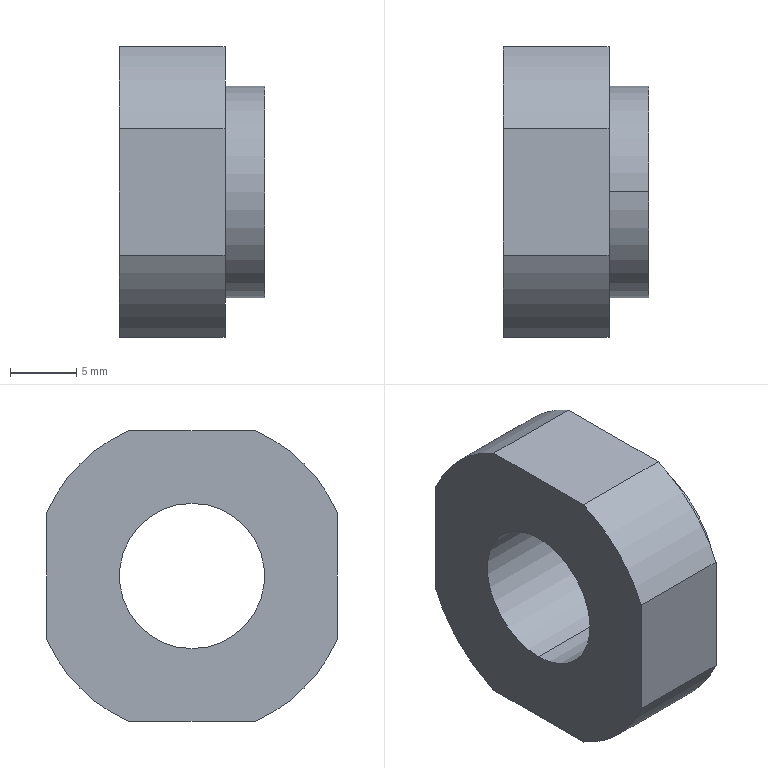Part | STEP file | PN_0032 locking nut | 1 solid | 15 faces | box 11 x 22 x 22 mm | volume 2971 mm3 | cylinder 8 | plane 7 | commonest cylinder face diameters 24 x4 11 x2 16 x2
STEP:
#1=CARTESIAN_POINT('',(0.,0.,0.));
#2=DIRECTION('',(0.,0.,1.));
#3=DIRECTION('',(1.,0.,0.));
#4=AXIS2_PLACEMENT_3D('',#1,#2,#3);
#5=CARTESIAN_POINT('',(-11.,0.,-5.5));
#6=VERTEX_POINT('',#5);
#7=CARTESIAN_POINT('',(0.,0.,-5.5));
#8=VERTEX_POINT('',#7);
#9=CARTESIAN_POINT('',(-11.,0.,-5.5));
#10=DIRECTION('',(1.,0.,0.));
#11=VECTOR('',#10,1.);
#12=LINE('',#9,#11);
#13=CARTESIAN_POINT('',(-11.,0.,0.));
#14=DIRECTION('',(1.,0.,0.));
#15=DIRECTION('',(0.,0.,-1.));
#16=AXIS2_PLACEMENT_3D('',#13,#14,#15);
#17=CYLINDRICAL_SURFACE('',#16,5.5);
#18=CARTESIAN_POINT('',(6.283,0.));
#19=DIRECTION('',(0.,1.));
#20=VECTOR('',#19,1.);
#21=LINE('',#18,#20);
#22=(GEOMETRIC_REPRESENTATION_CONTEXT(2)PARAMETRIC_REPRESENTATION_CONTEXT()REPRESENTATION_CONTEXT('',''));
#23=DEFINITIONAL_REPRESENTATION('',(#21),#22);
#24=PCURVE('',#17,#23);
#25=CARTESIAN_POINT('',(-11.,0.,0.));
#26=DIRECTION('',(1.,0.,0.));
#27=DIRECTION('',(0.,0.,-1.));
#28=AXIS2_PLACEMENT_3D('',#25,#26,#27);
#29=CYLINDRICAL_SURFACE('',#28,5.5);
#30=CARTESIAN_POINT('',(0.,0.));
#31=DIRECTION('',(0.,1.));
#32=VECTOR('',#31,1.);
#33=LINE('',#30,#32);
#34=(GEOMETRIC_REPRESENTATION_CONTEXT(2)PARAMETRIC_REPRESENTATION_CONTEXT()REPRESENTATION_CONTEXT('',''));
#35=DEFINITIONAL_REPRESENTATION('',(#33),#34);
#36=PCURVE('',#29,#35);
#37=SURFACE_CURVE('',#12,(#24,#36),.PCURVE_S1.);
#38=EDGE_CURVE('',#6,#8,#37,.T.);
#39=ORIENTED_EDGE('',*,*,#38,.T.);
#40=CARTESIAN_POINT('',(0.,0.,5.5));
#41=VERTEX_POINT('',#40);
#42=CARTESIAN_POINT('',(0.,0.,0.));
#43=DIRECTION('',(1.,0.,0.));
#44=DIRECTION('',(0.,0.,-1.));
#45=AXIS2_PLACEMENT_3D('',#42,#43,#44);
#46=CIRCLE('',#45,5.5);
#47=CARTESIAN_POINT('',(0.,11.));
#48=DIRECTION('',(1.,0.));
#49=VECTOR('',#48,1.);
#50=LINE('',#47,#49);
#51=(GEOMETRIC_REPRESENTATION_CONTEXT(2)PARAMETRIC_REPRESENTATION_CONTEXT()REPRESENTATION_CONTEXT('',''));
#52=DEFINITIONAL_REPRESENTATION('',(#50),#51);
#53=PCURVE('',#17,#52);
#54=CARTESIAN_POINT('',(0.,0.,0.));
#55=DIRECTION('',(1.,0.,0.));
#56=DIRECTION('',(0.,0.,-1.));
#57=AXIS2_PLACEMENT_3D('',#54,#55,#56);
#58=PLANE('',#57);
#59=CARTESIAN_POINT('',(0.,0.));
#60=DIRECTION('',(1.,0.));
#61=AXIS2_PLACEMENT_2D('',#59,#60);
#62=CIRCLE('',#61,5.5);
#63=(GEOMETRIC_REPRESENTATION_CONTEXT(2)PARAMETRIC_REPRESENTATION_CONTEXT()REPRESENTATION_CONTEXT('',''));
#64=DEFINITIONAL_REPRESENTATION('',(#62),#63);
#65=PCURVE('',#58,#64);
#66=SURFACE_CURVE('',#46,(#53,#65),.PCURVE_S1.);
#67=EDGE_CURVE('',#41,#8,#66,.T.);
#68=ORIENTED_EDGE('',*,*,#67,.F.);
#69=CARTESIAN_POINT('',(-11.,0.,5.5));
#70=VERTEX_POINT('',#69);
#71=CARTESIAN_POINT('',(-11.,0.,5.5));
#72=DIRECTION('',(1.,0.,0.));
#73=VECTOR('',#72,1.);
#74=LINE('',#71,#73);
#75=CARTESIAN_POINT('',(3.142,0.));
#76=DIRECTION('',(0.,1.));
#77=VECTOR('',#76,1.);
#78=LINE('',#75,#77);
#79=(GEOMETRIC_REPRESENTATION_CONTEXT(2)PARAMETRIC_REPRESENTATION_CONTEXT()REPRESENTATION_CONTEXT('',''));
#80=DEFINITIONAL_REPRESENTATION('',(#78),#79);
#81=PCURVE('',#17,#80);
#82=CARTESIAN_POINT('',(3.142,0.));
#83=DIRECTION('',(0.,1.));
#84=VECTOR('',#83,1.);
#85=LINE('',#82,#84);
#86=(GEOMETRIC_REPRESENTATION_CONTEXT(2)PARAMETRIC_REPRESENTATION_CONTEXT()REPRESENTATION_CONTEXT('',''));
#87=DEFINITIONAL_REPRESENTATION('',(#85),#86);
#88=PCURVE('',#29,#87);
#89=SURFACE_CURVE('',#74,(#81,#88),.PCURVE_S1.);
#90=EDGE_CURVE('',#70,#41,#89,.T.);
#91=ORIENTED_EDGE('',*,*,#90,.F.);
#92=CARTESIAN_POINT('',(-11.,0.,0.));
#93=DIRECTION('',(1.,0.,0.));
#94=DIRECTION('',(0.,0.,-1.));
#95=AXIS2_PLACEMENT_3D('',#92,#93,#94);
#96=CIRCLE('',#95,5.5);
#97=CARTESIAN_POINT('',(0.,0.));
#98=DIRECTION('',(1.,0.));
#99=VECTOR('',#98,1.);
#100=LINE('',#97,#99);
#101=(GEOMETRIC_REPRESENTATION_CONTEXT(2)PARAMETRIC_REPRESENTATION_CONTEXT()REPRESENTATION_CONTEXT('',''));
#102=DEFINITIONAL_REPRESENTATION('',(#100),#101);
#103=PCURVE('',#17,#102);
#104=CARTESIAN_POINT('',(-11.,12.,0.));
#105=DIRECTION('',(-1.,0.,0.));
#106=DIRECTION('',(0.,0.,1.));
#107=AXIS2_PLACEMENT_3D('',#104,#105,#106);
#108=PLANE('',#107);
#109=CARTESIAN_POINT('',(-5.5,-12.));
#110=CARTESIAN_POINT('',(-5.5,-2.474));
#111=CARTESIAN_POINT('',(2.75,-7.237));
#112=CARTESIAN_POINT('',(11.,-12.));
#113=CARTESIAN_POINT('',(2.75,-16.763));
#114=CARTESIAN_POINT('',(-5.5,-21.526));
#115=CARTESIAN_POINT('',(-5.5,-12.));
#116=(BOUNDED_CURVE()B_SPLINE_CURVE(2,(#109,#110,#111,#112,#113,#114,#115),.UNSPECIFIED.,.T.,.F.)B_SPLINE_CURVE_WITH_KNOTS((1,2,2,2,2,1),(-2.094,0.,2.094,4.189,6.283,8.378),.UNSPECIFIED.)CURVE()GEOMETRIC_REPRESENTATION_ITEM()RATIONAL_B_SPLINE_CURVE((1.,0.5,1.,0.5,1.,0.5,1.))REPRESENTATION_ITEM(''));
#117=(GEOMETRIC_REPRESENTATION_CONTEXT(2)PARAMETRIC_REPRESENTATION_CONTEXT()REPRESENTATION_CONTEXT('',''));
#118=DEFINITIONAL_REPRESENTATION('',(#116),#117);
#119=PCURVE('',#108,#118);
#120=SURFACE_CURVE('',#96,(#103,#119),.PCURVE_S1.);
#121=EDGE_CURVE('',#70,#6,#120,.T.);
#122=ORIENTED_EDGE('',*,*,#121,.T.);
#123=EDGE_LOOP('',(#39,#68,#91,#122));
#124=FACE_BOUND('',#123,.F.);
#125=ADVANCED_FACE('',(#124),#17,.F.);
#126=CARTESIAN_POINT('',(-3.,0.,-8.));
#127=VERTEX_POINT('',#126);
#128=CARTESIAN_POINT('',(-3.,0.,8.));
#129=VERTEX_POINT('',#128);
#130=CARTESIAN_POINT('',(-3.,0.,0.));
#131=DIRECTION('',(1.,0.,0.));
#132=DIRECTION('',(0.,0.,-1.));
#133=AXIS2_PLACEMENT_3D('',#130,#131,#132);
#134=CIRCLE('',#133,8.);
#135=CARTESIAN_POINT('',(0.,0.,0.));
#136=DIRECTION('',(1.,0.,0.));
#137=DIRECTION('',(0.,0.,-1.));
#138=AXIS2_PLACEMENT_3D('',#135,#136,#137);
#139=CYLINDRICAL_SURFACE('',#138,8.);
#140=CARTESIAN_POINT('',(0.,-3.));
#141=DIRECTION('',(1.,0.));
#142=VECTOR('',#141,1.);
#143=LINE('',#140,#142);
#144=(GEOMETRIC_REPRESENTATION_CONTEXT(2)PARAMETRIC_REPRESENTATION_CONTEXT()REPRESENTATION_CONTEXT('',''));
#145=DEFINITIONAL_REPRESENTATION('',(#143),#144);
#146=PCURVE('',#139,#145);
#147=CARTESIAN_POINT('',(-3.,8.,0.));
#148=DIRECTION('',(1.,0.,0.));
#149=DIRECTION('',(0.,0.,-1.));
#150=AXIS2_PLACEMENT_3D('',#147,#148,#149);
#151=PLANE('',#150);
#152=CARTESIAN_POINT('',(0.,-8.));
#153=DIRECTION('',(1.,0.));
#154=AXIS2_PLACEMENT_2D('',#152,#153);
#155=CIRCLE('',#154,8.);
#156=(GEOMETRIC_REPRESENTATION_CONTEXT(2)PARAMETRIC_REPRESENTATION_CONTEXT()REPRESENTATION_CONTEXT('',''));
#157=DEFINITIONAL_REPRESENTATION('',(#155),#156);
#158=PCURVE('',#151,#157);
#159=SURFACE_CURVE('',#134,(#146,#158),.PCURVE_S1.);
#160=EDGE_CURVE('',#127,#129,#159,.T.);
#161=ORIENTED_EDGE('',*,*,#160,.T.);
#162=CARTESIAN_POINT('',(0.,0.,8.));
#163=VERTEX_POINT('',#162);
#164=CARTESIAN_POINT('',(0.,0.,8.));
#165=DIRECTION('',(1.,0.,0.));
#166=VECTOR('',#165,1.);
#167=LINE('',#164,#166);
#168=CARTESIAN_POINT('',(3.142,0.));
#169=DIRECTION('',(0.,1.));
#170=VECTOR('',#169,1.);
#171=LINE('',#168,#170);
#172=(GEOMETRIC_REPRESENTATION_CONTEXT(2)PARAMETRIC_REPRESENTATION_CONTEXT()REPRESENTATION_CONTEXT('',''));
#173=DEFINITIONAL_REPRESENTATION('',(#171),#172);
#174=PCURVE('',#139,#173);
#175=CARTESIAN_POINT('',(0.,0.,0.));
#176=DIRECTION('',(1.,0.,0.));
#177=DIRECTION('',(0.,0.,-1.));
#178=AXIS2_PLACEMENT_3D('',#175,#176,#177);
#179=CYLINDRICAL_SURFACE('',#178,8.);
#180=CARTESIAN_POINT('',(3.142,0.));
#181=DIRECTION('',(0.,1.));
#182=VECTOR('',#181,1.);
#183=LINE('',#180,#182);
#184=(GEOMETRIC_REPRESENTATION_CONTEXT(2)PARAMETRIC_REPRESENTATION_CONTEXT()REPRESENTATION_CONTEXT('',''));
#185=DEFINITIONAL_REPRESENTATION('',(#183),#184);
#186=PCURVE('',#179,#185);
#187=SURFACE_CURVE('',#167,(#174,#186),.PCURVE_S1.);
#188=EDGE_CURVE('',#129,#163,#187,.T.);
#189=ORIENTED_EDGE('',*,*,#188,.T.);
#190=CARTESIAN_POINT('',(0.,0.,-8.));
#191=VERTEX_POINT('',#190);
#192=CARTESIAN_POINT('',(0.,0.,0.));
#193=DIRECTION('',(1.,0.,0.));
#194=DIRECTION('',(0.,0.,-1.));
#195=AXIS2_PLACEMENT_3D('',#192,#193,#194);
#196=CIRCLE('',#195,8.);
#197=CARTESIAN_POINT('',(0.,0.));
#198=DIRECTION('',(1.,0.));
#199=VECTOR('',#198,1.);
#200=LINE('',#197,#199);
#201=(GEOMETRIC_REPRESENTATION_CONTEXT(2)PARAMETRIC_REPRESENTATION_CONTEXT()REPRESENTATION_CONTEXT('',''));
#202=DEFINITIONAL_REPRESENTATION('',(#200),#201);
#203=PCURVE('',#139,#202);
#204=CARTESIAN_POINT('',(0.,0.));
#205=DIRECTION('',(1.,0.));
#206=AXIS2_PLACEMENT_2D('',#204,#205);
#207=CIRCLE('',#206,8.);
#208=(GEOMETRIC_REPRESENTATION_CONTEXT(2)PARAMETRIC_REPRESENTATION_CONTEXT()REPRESENTATION_CONTEXT('',''));
#209=DEFINITIONAL_REPRESENTATION('',(#207),#208);
#210=PCURVE('',#58,#209);
#211=SURFACE_CURVE('',#196,(#203,#210),.PCURVE_S1.);
#212=EDGE_CURVE('',#191,#163,#211,.T.);
#213=ORIENTED_EDGE('',*,*,#212,.F.);
#214=CARTESIAN_POINT('',(0.,0.,-8.));
#215=DIRECTION('',(1.,0.,0.));
#216=VECTOR('',#215,1.);
#217=LINE('',#214,#216);
#218=CARTESIAN_POINT('',(0.,0.));
#219=DIRECTION('',(0.,1.));
#220=VECTOR('',#219,1.);
#221=LINE('',#218,#220);
#222=(GEOMETRIC_REPRESENTATION_CONTEXT(2)PARAMETRIC_REPRESENTATION_CONTEXT()REPRESENTATION_CONTEXT('',''));
#223=DEFINITIONAL_REPRESENTATION('',(#221),#222);
#224=PCURVE('',#139,#223);
#225=CARTESIAN_POINT('',(6.283,0.));
#226=DIRECTION('',(0.,1.));
#227=VECTOR('',#226,1.);
#228=LINE('',#225,#227);
#229=(GEOMETRIC_REPRESENTATION_CONTEXT(2)PARAMETRIC_REPRESENTATION_CONTEXT()REPRESENTATION_CONTEXT('',''));
#230=DEFINITIONAL_REPRESENTATION('',(#228),#229);
#231=PCURVE('',#179,#230);
#232=SURFACE_CURVE('',#217,(#224,#231),.PCURVE_S1.);
#233=EDGE_CURVE('',#127,#191,#232,.T.);
#234=ORIENTED_EDGE('',*,*,#233,.F.);
#235=EDGE_LOOP('',(#161,#189,#213,#234));
#236=FACE_BOUND('',#235,.T.);
#237=ADVANCED_FACE('',(#236),#139,.T.);
#238=CARTESIAN_POINT('',(-3.,4.796,11.));
#239=VERTEX_POINT('',#238);
#240=CARTESIAN_POINT('',(-11.,4.796,11.));
#241=VERTEX_POINT('',#240);
#242=CARTESIAN_POINT('',(0.,4.796,11.));
#243=DIRECTION('',(-1.,0.,0.));
#244=VECTOR('',#243,1.);
#245=LINE('',#242,#244);
#246=CARTESIAN_POINT('',(0.,0.,0.));
#247=DIRECTION('',(1.,0.,0.));
#248=DIRECTION('',(0.,0.,-1.));
#249=AXIS2_PLACEMENT_3D('',#246,#247,#248);
#250=CYLINDRICAL_SURFACE('',#249,12.);
#251=CARTESIAN_POINT('',(2.73,0.));
#252=DIRECTION('',(0.,-1.));
#253=VECTOR('',#252,1.);
#254=LINE('',#251,#253);
#255=(GEOMETRIC_REPRESENTATION_CONTEXT(2)PARAMETRIC_REPRESENTATION_CONTEXT()REPRESENTATION_CONTEXT('',''));
#256=DEFINITIONAL_REPRESENTATION('',(#254),#255);
#257=PCURVE('',#250,#256);
#258=CARTESIAN_POINT('',(0.,17.205,11.));
#259=DIRECTION('',(0.,0.,-1.));
#260=DIRECTION('',(0.,1.,0.));
#261=AXIS2_PLACEMENT_3D('',#258,#259,#260);
#262=PLANE('',#261);
#263=CARTESIAN_POINT('',(-12.409,0.));
#264=DIRECTION('',(0.,-1.));
#265=VECTOR('',#264,1.);
#266=LINE('',#263,#265);
#267=(GEOMETRIC_REPRESENTATION_CONTEXT(2)PARAMETRIC_REPRESENTATION_CONTEXT()REPRESENTATION_CONTEXT('',''));
#268=DEFINITIONAL_REPRESENTATION('',(#266),#267);
#269=PCURVE('',#262,#268);
#270=SURFACE_CURVE('',#245,(#257,#269),.PCURVE_S1.);
#271=EDGE_CURVE('',#239,#241,#270,.T.);
#272=ORIENTED_EDGE('',*,*,#271,.F.);
#273=CARTESIAN_POINT('',(-3.,11.,4.796));
#274=VERTEX_POINT('',#273);
#275=CARTESIAN_POINT('',(-3.,0.,0.));
#276=DIRECTION('',(1.,0.,0.));
#277=DIRECTION('',(0.,0.,-1.));
#278=AXIS2_PLACEMENT_3D('',#275,#276,#277);
#279=CIRCLE('',#278,12.);
#280=CARTESIAN_POINT('',(0.,-3.));
#281=DIRECTION('',(1.,0.));
#282=VECTOR('',#281,1.);
#283=LINE('',#280,#282);
#284=(GEOMETRIC_REPRESENTATION_CONTEXT(2)PARAMETRIC_REPRESENTATION_CONTEXT()REPRESENTATION_CONTEXT('',''));
#285=DEFINITIONAL_REPRESENTATION('',(#283),#284);
#286=PCURVE('',#250,#285);
#287=CARTESIAN_POINT('',(0.,-8.));
#288=DIRECTION('',(1.,0.));
#289=AXIS2_PLACEMENT_2D('',#287,#288);
#290=CIRCLE('',#289,12.);
#291=(GEOMETRIC_REPRESENTATION_CONTEXT(2)PARAMETRIC_REPRESENTATION_CONTEXT()REPRESENTATION_CONTEXT('',''));
#292=DEFINITIONAL_REPRESENTATION('',(#290),#291);
#293=PCURVE('',#151,#292);
#294=SURFACE_CURVE('',#279,(#286,#293),.PCURVE_S1.);
#295=EDGE_CURVE('',#274,#239,#294,.T.);
#296=ORIENTED_EDGE('',*,*,#295,.F.);
#297=CARTESIAN_POINT('',(-11.,11.,4.796));
#298=VERTEX_POINT('',#297);
#299=CARTESIAN_POINT('',(0.,11.,4.796));
#300=DIRECTION('',(1.,0.,0.));
#301=VECTOR('',#300,1.);
#302=LINE('',#299,#301);
#303=CARTESIAN_POINT('',(1.982,0.));
#304=DIRECTION('',(0.,1.));
#305=VECTOR('',#304,1.);
#306=LINE('',#303,#305);
#307=(GEOMETRIC_REPRESENTATION_CONTEXT(2)PARAMETRIC_REPRESENTATION_CONTEXT()REPRESENTATION_CONTEXT('',''));
#308=DEFINITIONAL_REPRESENTATION('',(#306),#307);
#309=PCURVE('',#250,#308);
#310=CARTESIAN_POINT('',(0.,11.,-20.296));
#311=DIRECTION('',(0.,-1.,0.));
#312=DIRECTION('',(0.,0.,-1.));
#313=AXIS2_PLACEMENT_3D('',#310,#311,#312);
#314=PLANE('',#313);
#315=CARTESIAN_POINT('',(-25.092,0.));
#316=DIRECTION('',(0.,1.));
#317=VECTOR('',#316,1.);
#318=LINE('',#315,#317);
#319=(GEOMETRIC_REPRESENTATION_CONTEXT(2)PARAMETRIC_REPRESENTATION_CONTEXT()REPRESENTATION_CONTEXT('',''));
#320=DEFINITIONAL_REPRESENTATION('',(#318),#319);
#321=PCURVE('',#314,#320);
#322=SURFACE_CURVE('',#302,(#309,#321),.PCURVE_S1.);
#323=EDGE_CURVE('',#298,#274,#322,.T.);
#324=ORIENTED_EDGE('',*,*,#323,.F.);
#325=CARTESIAN_POINT('',(-11.,0.,0.));
#326=DIRECTION('',(1.,0.,0.));
#327=DIRECTION('',(0.,0.,-1.));
#328=AXIS2_PLACEMENT_3D('',#325,#326,#327);
#329=CIRCLE('',#328,12.);
#330=CARTESIAN_POINT('',(0.,-11.));
#331=DIRECTION('',(1.,0.));
#332=VECTOR('',#331,1.);
#333=LINE('',#330,#332);
#334=(GEOMETRIC_REPRESENTATION_CONTEXT(2)PARAMETRIC_REPRESENTATION_CONTEXT()REPRESENTATION_CONTEXT('',''));
#335=DEFINITIONAL_REPRESENTATION('',(#333),#334);
#336=PCURVE('',#250,#335);
#337=CARTESIAN_POINT('',(-12.,-12.));
#338=CARTESIAN_POINT('',(-12.,8.785));
#339=CARTESIAN_POINT('',(6.,-1.608));
#340=CARTESIAN_POINT('',(24.,-12.));
#341=CARTESIAN_POINT('',(6.,-22.392));
#342=CARTESIAN_POINT('',(-12.,-32.785));
#343=CARTESIAN_POINT('',(-12.,-12.));
#344=(BOUNDED_CURVE()B_SPLINE_CURVE(2,(#337,#338,#339,#340,#341,#342,#343),.UNSPECIFIED.,.T.,.F.)B_SPLINE_CURVE_WITH_KNOTS((1,2,2,2,2,1),(-2.094,0.,2.094,4.189,6.283,8.378),.UNSPECIFIED.)CURVE()GEOMETRIC_REPRESENTATION_ITEM()RATIONAL_B_SPLINE_CURVE((1.,0.5,1.,0.5,1.,0.5,1.))REPRESENTATION_ITEM(''));
#345=(GEOMETRIC_REPRESENTATION_CONTEXT(2)PARAMETRIC_REPRESENTATION_CONTEXT()REPRESENTATION_CONTEXT('',''));
#346=DEFINITIONAL_REPRESENTATION('',(#344),#345);
#347=PCURVE('',#108,#346);
#348=SURFACE_CURVE('',#329,(#336,#347),.PCURVE_S1.);
#349=EDGE_CURVE('',#298,#241,#348,.T.);
#350=ORIENTED_EDGE('',*,*,#349,.T.);
#351=EDGE_LOOP('',(#272,#296,#324,#350));
#352=FACE_BOUND('',#351,.T.);
#353=ADVANCED_FACE('',(#352),#250,.T.);
#354=CARTESIAN_POINT('',(-3.,-4.796,-11.));
#355=VERTEX_POINT('',#354);
#356=CARTESIAN_POINT('',(-11.,-4.796,-11.));
#357=VERTEX_POINT('',#356);
#358=CARTESIAN_POINT('',(0.,-4.796,-11.));
#359=DIRECTION('',(-1.,0.,0.));
#360=VECTOR('',#359,1.);
#361=LINE('',#358,#360);
#362=CARTESIAN_POINT('',(0.,0.,0.));
#363=DIRECTION('',(1.,0.,0.));
#364=DIRECTION('',(0.,0.,-1.));
#365=AXIS2_PLACEMENT_3D('',#362,#363,#364);
#366=CYLINDRICAL_SURFACE('',#365,12.);
#367=CARTESIAN_POINT('',(5.872,0.));
#368=DIRECTION('',(0.,-1.));
#369=VECTOR('',#368,1.);
#370=LINE('',#367,#369);
#371=(GEOMETRIC_REPRESENTATION_CONTEXT(2)PARAMETRIC_REPRESENTATION_CONTEXT()REPRESENTATION_CONTEXT('',''));
#372=DEFINITIONAL_REPRESENTATION('',(#370),#371);
#373=PCURVE('',#366,#372);
#374=CARTESIAN_POINT('',(0.,17.205,-11.));
#375=DIRECTION('',(0.,0.,1.));
#376=DIRECTION('',(0.,-1.,0.));
#377=AXIS2_PLACEMENT_3D('',#374,#375,#376);
#378=PLANE('',#377);
#379=CARTESIAN_POINT('',(22.001,0.));
#380=DIRECTION('',(0.,-1.));
#381=VECTOR('',#380,1.);
#382=LINE('',#379,#381);
#383=(GEOMETRIC_REPRESENTATION_CONTEXT(2)PARAMETRIC_REPRESENTATION_CONTEXT()REPRESENTATION_CONTEXT('',''));
#384=DEFINITIONAL_REPRESENTATION('',(#382),#383);
#385=PCURVE('',#378,#384);
#386=SURFACE_CURVE('',#361,(#373,#385),.PCURVE_S1.);
#387=EDGE_CURVE('',#355,#357,#386,.T.);
#388=ORIENTED_EDGE('',*,*,#387,.F.);
#389=CARTESIAN_POINT('',(-3.,-11.,-4.796));
#390=VERTEX_POINT('',#389);
#391=CARTESIAN_POINT('',(-3.,0.,0.));
#392=DIRECTION('',(1.,0.,0.));
#393=DIRECTION('',(0.,0.,-1.));
#394=AXIS2_PLACEMENT_3D('',#391,#392,#393);
#395=CIRCLE('',#394,12.);
#396=CARTESIAN_POINT('',(0.,-3.));
#397=DIRECTION('',(1.,0.));
#398=VECTOR('',#397,1.);
#399=LINE('',#396,#398);
#400=(GEOMETRIC_REPRESENTATION_CONTEXT(2)PARAMETRIC_REPRESENTATION_CONTEXT()REPRESENTATION_CONTEXT('',''));
#401=DEFINITIONAL_REPRESENTATION('',(#399),#400);
#402=PCURVE('',#366,#401);
#403=CARTESIAN_POINT('',(0.,-8.));
#404=DIRECTION('',(1.,0.));
#405=AXIS2_PLACEMENT_2D('',#403,#404);
#406=CIRCLE('',#405,12.);
#407=(GEOMETRIC_REPRESENTATION_CONTEXT(2)PARAMETRIC_REPRESENTATION_CONTEXT()REPRESENTATION_CONTEXT('',''));
#408=DEFINITIONAL_REPRESENTATION('',(#406),#407);
#409=PCURVE('',#151,#408);
#410=SURFACE_CURVE('',#395,(#402,#409),.PCURVE_S1.);
#411=EDGE_CURVE('',#390,#355,#410,.T.);
#412=ORIENTED_EDGE('',*,*,#411,.F.);
#413=CARTESIAN_POINT('',(-11.,-11.,-4.796));
#414=VERTEX_POINT('',#413);
#415=CARTESIAN_POINT('',(0.,-11.,-4.796));
#416=DIRECTION('',(1.,0.,0.));
#417=VECTOR('',#416,1.);
#418=LINE('',#415,#417);
#419=CARTESIAN_POINT('',(5.124,0.));
#420=DIRECTION('',(0.,1.));
#421=VECTOR('',#420,1.);
#422=LINE('',#419,#421);
#423=(GEOMETRIC_REPRESENTATION_CONTEXT(2)PARAMETRIC_REPRESENTATION_CONTEXT()REPRESENTATION_CONTEXT('',''));
#424=DEFINITIONAL_REPRESENTATION('',(#422),#423);
#425=PCURVE('',#366,#424);
#426=CARTESIAN_POINT('',(0.,-11.,-20.296));
#427=DIRECTION('',(0.,1.,0.));
#428=DIRECTION('',(0.,0.,1.));
#429=AXIS2_PLACEMENT_3D('',#426,#427,#428);
#430=PLANE('',#429);
#431=CARTESIAN_POINT('',(15.501,0.));
#432=DIRECTION('',(0.,1.));
#433=VECTOR('',#432,1.);
#434=LINE('',#431,#433);
#435=(GEOMETRIC_REPRESENTATION_CONTEXT(2)PARAMETRIC_REPRESENTATION_CONTEXT()REPRESENTATION_CONTEXT('',''));
#436=DEFINITIONAL_REPRESENTATION('',(#434),#435);
#437=PCURVE('',#430,#436);
#438=SURFACE_CURVE('',#418,(#425,#437),.PCURVE_S1.);
#439=EDGE_CURVE('',#414,#390,#438,.T.);
#440=ORIENTED_EDGE('',*,*,#439,.F.);
#441=CARTESIAN_POINT('',(-11.,0.,0.));
#442=DIRECTION('',(1.,0.,0.));
#443=DIRECTION('',(0.,0.,-1.));
#444=AXIS2_PLACEMENT_3D('',#441,#442,#443);
#445=CIRCLE('',#444,12.);
#446=CARTESIAN_POINT('',(0.,-11.));
#447=DIRECTION('',(1.,0.));
#448=VECTOR('',#447,1.);
#449=LINE('',#446,#448);
#450=(GEOMETRIC_REPRESENTATION_CONTEXT(2)PARAMETRIC_REPRESENTATION_CONTEXT()REPRESENTATION_CONTEXT('',''));
#451=DEFINITIONAL_REPRESENTATION('',(#449),#450);
#452=PCURVE('',#366,#451);
#453=CARTESIAN_POINT('',(-12.,-12.));
#454=CARTESIAN_POINT('',(-12.,8.785));
#455=CARTESIAN_POINT('',(6.,-1.608));
#456=CARTESIAN_POINT('',(24.,-12.));
#457=CARTESIAN_POINT('',(6.,-22.392));
#458=CARTESIAN_POINT('',(-12.,-32.785));
#459=CARTESIAN_POINT('',(-12.,-12.));
#460=(BOUNDED_CURVE()B_SPLINE_CURVE(2,(#453,#454,#455,#456,#457,#458,#459),.UNSPECIFIED.,.T.,.F.)B_SPLINE_CURVE_WITH_KNOTS((1,2,2,2,2,1),(-2.094,0.,2.094,4.189,6.283,8.378),.UNSPECIFIED.)CURVE()GEOMETRIC_REPRESENTATION_ITEM()RATIONAL_B_SPLINE_CURVE((1.,0.5,1.,0.5,1.,0.5,1.))REPRESENTATION_ITEM(''));
#461=(GEOMETRIC_REPRESENTATION_CONTEXT(2)PARAMETRIC_REPRESENTATION_CONTEXT()REPRESENTATION_CONTEXT('',''));
#462=DEFINITIONAL_REPRESENTATION('',(#460),#461);
#463=PCURVE('',#108,#462);
#464=SURFACE_CURVE('',#445,(#452,#463),.PCURVE_S1.);
#465=EDGE_CURVE('',#414,#357,#464,.T.);
#466=ORIENTED_EDGE('',*,*,#465,.T.);
#467=EDGE_LOOP('',(#388,#412,#440,#466));
#468=FACE_BOUND('',#467,.T.);
#469=ADVANCED_FACE('',(#468),#366,.T.);
#470=CARTESIAN_POINT('',(-11.,-4.796,11.));
#471=VERTEX_POINT('',#470);
#472=CARTESIAN_POINT('',(-3.,-4.796,11.));
#473=VERTEX_POINT('',#472);
#474=CARTESIAN_POINT('',(0.,-4.796,11.));
#475=DIRECTION('',(1.,0.,0.));
#476=VECTOR('',#475,1.);
#477=LINE('',#474,#476);
#478=CARTESIAN_POINT('',(0.,0.,0.));
#479=DIRECTION('',(1.,0.,0.));
#480=DIRECTION('',(0.,0.,-1.));
#481=AXIS2_PLACEMENT_3D('',#478,#479,#480);
#482=CYLINDRICAL_SURFACE('',#481,12.);
#483=CARTESIAN_POINT('',(3.553,0.));
#484=DIRECTION('',(0.,1.));
#485=VECTOR('',#484,1.);
#486=LINE('',#483,#485);
#487=(GEOMETRIC_REPRESENTATION_CONTEXT(2)PARAMETRIC_REPRESENTATION_CONTEXT()REPRESENTATION_CONTEXT('',''));
#488=DEFINITIONAL_REPRESENTATION('',(#486),#487);
#489=PCURVE('',#482,#488);
#490=CARTESIAN_POINT('',(-22.001,0.));
#491=DIRECTION('',(0.,1.));
#492=VECTOR('',#491,1.);
#493=LINE('',#490,#492);
#494=(GEOMETRIC_REPRESENTATION_CONTEXT(2)PARAMETRIC_REPRESENTATION_CONTEXT()REPRESENTATION_CONTEXT('',''));
#495=DEFINITIONAL_REPRESENTATION('',(#493),#494);
#496=PCURVE('',#262,#495);
#497=SURFACE_CURVE('',#477,(#489,#496),.PCURVE_S1.);
#498=EDGE_CURVE('',#471,#473,#497,.T.);
#499=ORIENTED_EDGE('',*,*,#498,.F.);
#500=CARTESIAN_POINT('',(-11.,-11.,4.796));
#501=VERTEX_POINT('',#500);
#502=CARTESIAN_POINT('',(-11.,0.,0.));
#503=DIRECTION('',(1.,0.,0.));
#504=DIRECTION('',(0.,0.,-1.));
#505=AXIS2_PLACEMENT_3D('',#502,#503,#504);
#506=CIRCLE('',#505,12.);
#507=CARTESIAN_POINT('',(0.,-11.));
#508=DIRECTION('',(1.,0.));
#509=VECTOR('',#508,1.);
#510=LINE('',#507,#509);
#511=(GEOMETRIC_REPRESENTATION_CONTEXT(2)PARAMETRIC_REPRESENTATION_CONTEXT()REPRESENTATION_CONTEXT('',''));
#512=DEFINITIONAL_REPRESENTATION('',(#510),#511);
#513=PCURVE('',#482,#512);
#514=CARTESIAN_POINT('',(-12.,-12.));
#515=CARTESIAN_POINT('',(-12.,8.785));
#516=CARTESIAN_POINT('',(6.,-1.608));
#517=CARTESIAN_POINT('',(24.,-12.));
#518=CARTESIAN_POINT('',(6.,-22.392));
#519=CARTESIAN_POINT('',(-12.,-32.785));
#520=CARTESIAN_POINT('',(-12.,-12.));
#521=(BOUNDED_CURVE()B_SPLINE_CURVE(2,(#514,#515,#516,#517,#518,#519,#520),.UNSPECIFIED.,.T.,.F.)B_SPLINE_CURVE_WITH_KNOTS((1,2,2,2,2,1),(-2.094,0.,2.094,4.189,6.283,8.378),.UNSPECIFIED.)CURVE()GEOMETRIC_REPRESENTATION_ITEM()RATIONAL_B_SPLINE_CURVE((1.,0.5,1.,0.5,1.,0.5,1.))REPRESENTATION_ITEM(''));
#522=(GEOMETRIC_REPRESENTATION_CONTEXT(2)PARAMETRIC_REPRESENTATION_CONTEXT()REPRESENTATION_CONTEXT('',''));
#523=DEFINITIONAL_REPRESENTATION('',(#521),#522);
#524=PCURVE('',#108,#523);
#525=SURFACE_CURVE('',#506,(#513,#524),.PCURVE_S1.);
#526=EDGE_CURVE('',#471,#501,#525,.T.);
#527=ORIENTED_EDGE('',*,*,#526,.T.);
#528=CARTESIAN_POINT('',(-3.,-11.,4.796));
#529=VERTEX_POINT('',#528);
#530=CARTESIAN_POINT('',(0.,-11.,4.796));
#531=DIRECTION('',(-1.,0.,0.));
#532=VECTOR('',#531,1.);
#533=LINE('',#530,#532);
#534=CARTESIAN_POINT('',(4.301,0.));
#535=DIRECTION('',(0.,-1.));
#536=VECTOR('',#535,1.);
#537=LINE('',#534,#536);
#538=(GEOMETRIC_REPRESENTATION_CONTEXT(2)PARAMETRIC_REPRESENTATION_CONTEXT()REPRESENTATION_CONTEXT('',''));
#539=DEFINITIONAL_REPRESENTATION('',(#537),#538);
#540=PCURVE('',#482,#539);
#541=CARTESIAN_POINT('',(25.092,0.));
#542=DIRECTION('',(0.,-1.));
#543=VECTOR('',#542,1.);
#544=LINE('',#541,#543);
#545=(GEOMETRIC_REPRESENTATION_CONTEXT(2)PARAMETRIC_REPRESENTATION_CONTEXT()REPRESENTATION_CONTEXT('',''));
#546=DEFINITIONAL_REPRESENTATION('',(#544),#545);
#547=PCURVE('',#430,#546);
#548=SURFACE_CURVE('',#533,(#540,#547),.PCURVE_S1.);
#549=EDGE_CURVE('',#529,#501,#548,.T.);
#550=ORIENTED_EDGE('',*,*,#549,.F.);
#551=CARTESIAN_POINT('',(-3.,0.,0.));
#552=DIRECTION('',(1.,0.,0.));
#553=DIRECTION('',(0.,0.,-1.));
#554=AXIS2_PLACEMENT_3D('',#551,#552,#553);
#555=CIRCLE('',#554,12.);
#556=CARTESIAN_POINT('',(0.,-3.));
#557=DIRECTION('',(1.,0.));
#558=VECTOR('',#557,1.);
#559=LINE('',#556,#558);
#560=(GEOMETRIC_REPRESENTATION_CONTEXT(2)PARAMETRIC_REPRESENTATION_CONTEXT()REPRESENTATION_CONTEXT('',''));
#561=DEFINITIONAL_REPRESENTATION('',(#559),#560);
#562=PCURVE('',#482,#561);
#563=CARTESIAN_POINT('',(0.,-8.));
#564=DIRECTION('',(1.,0.));
#565=AXIS2_PLACEMENT_2D('',#563,#564);
#566=CIRCLE('',#565,12.);
#567=(GEOMETRIC_REPRESENTATION_CONTEXT(2)PARAMETRIC_REPRESENTATION_CONTEXT()REPRESENTATION_CONTEXT('',''));
#568=DEFINITIONAL_REPRESENTATION('',(#566),#567);
#569=PCURVE('',#151,#568);
#570=SURFACE_CURVE('',#555,(#562,#569),.PCURVE_S1.);
#571=EDGE_CURVE('',#473,#529,#570,.T.);
#572=ORIENTED_EDGE('',*,*,#571,.F.);
#573=EDGE_LOOP('',(#499,#527,#550,#572));
#574=FACE_BOUND('',#573,.T.);
#575=ADVANCED_FACE('',(#574),#482,.T.);
#576=CARTESIAN_POINT('',(0.,0.,0.));
#577=DIRECTION('',(1.,0.,0.));
#578=DIRECTION('',(0.,0.,-1.));
#579=AXIS2_PLACEMENT_3D('',#576,#577,#578);
#580=CIRCLE('',#579,5.5);
#581=CARTESIAN_POINT('',(0.,0.));
#582=DIRECTION('',(1.,0.));
#583=AXIS2_PLACEMENT_2D('',#581,#582);
#584=CIRCLE('',#583,5.5);
#585=(GEOMETRIC_REPRESENTATION_CONTEXT(2)PARAMETRIC_REPRESENTATION_CONTEXT()REPRESENTATION_CONTEXT('',''));
#586=DEFINITIONAL_REPRESENTATION('',(#584),#585);
#587=PCURVE('',#58,#586);
#588=CARTESIAN_POINT('',(0.,11.));
#589=DIRECTION('',(1.,0.));
#590=VECTOR('',#589,1.);
#591=LINE('',#588,#590);
#592=(GEOMETRIC_REPRESENTATION_CONTEXT(2)PARAMETRIC_REPRESENTATION_CONTEXT()REPRESENTATION_CONTEXT('',''));
#593=DEFINITIONAL_REPRESENTATION('',(#591),#592);
#594=PCURVE('',#29,#593);
#595=SURFACE_CURVE('',#580,(#587,#594),.PCURVE_S1.);
#596=EDGE_CURVE('',#8,#41,#595,.T.);
#597=ORIENTED_EDGE('',*,*,#596,.F.);
#598=ORIENTED_EDGE('',*,*,#67,.F.);
#599=EDGE_LOOP('',(#597,#598));
#600=FACE_BOUND('',#599,.T.);
#601=ORIENTED_EDGE('',*,*,#212,.T.);
#602=CARTESIAN_POINT('',(0.,0.,0.));
#603=DIRECTION('',(1.,0.,0.));
#604=DIRECTION('',(0.,0.,-1.));
#605=AXIS2_PLACEMENT_3D('',#602,#603,#604);
#606=CIRCLE('',#605,8.);
#607=CARTESIAN_POINT('',(0.,0.));
#608=DIRECTION('',(1.,0.));
#609=AXIS2_PLACEMENT_2D('',#607,#608);
#610=CIRCLE('',#609,8.);
#611=(GEOMETRIC_REPRESENTATION_CONTEXT(2)PARAMETRIC_REPRESENTATION_CONTEXT()REPRESENTATION_CONTEXT('',''));
#612=DEFINITIONAL_REPRESENTATION('',(#610),#611);
#613=PCURVE('',#58,#612);
#614=CARTESIAN_POINT('',(0.,0.));
#615=DIRECTION('',(1.,0.));
#616=VECTOR('',#615,1.);
#617=LINE('',#614,#616);
#618=(GEOMETRIC_REPRESENTATION_CONTEXT(2)PARAMETRIC_REPRESENTATION_CONTEXT()REPRESENTATION_CONTEXT('',''));
#619=DEFINITIONAL_REPRESENTATION('',(#617),#618);
#620=PCURVE('',#179,#619);
#621=SURFACE_CURVE('',#606,(#613,#620),.PCURVE_S1.);
#622=EDGE_CURVE('',#163,#191,#621,.T.);
#623=ORIENTED_EDGE('',*,*,#622,.T.);
#624=EDGE_LOOP('',(#601,#623));
#625=FACE_BOUND('',#624,.T.);
#626=ADVANCED_FACE('',(#600,#625),#58,.T.);
#627=ORIENTED_EDGE('',*,*,#188,.F.);
#628=CARTESIAN_POINT('',(-3.,0.,0.));
#629=DIRECTION('',(1.,0.,0.));
#630=DIRECTION('',(0.,0.,-1.));
#631=AXIS2_PLACEMENT_3D('',#628,#629,#630);
#632=CIRCLE('',#631,8.);
#633=CARTESIAN_POINT('',(0.,-3.));
#634=DIRECTION('',(1.,0.));
#635=VECTOR('',#634,1.);
#636=LINE('',#633,#635);
#637=(GEOMETRIC_REPRESENTATION_CONTEXT(2)PARAMETRIC_REPRESENTATION_CONTEXT()REPRESENTATION_CONTEXT('',''));
#638=DEFINITIONAL_REPRESENTATION('',(#636),#637);
#639=PCURVE('',#179,#638);
#640=CARTESIAN_POINT('',(0.,-8.));
#641=DIRECTION('',(1.,0.));
#642=AXIS2_PLACEMENT_2D('',#640,#641);
#643=CIRCLE('',#642,8.);
#644=(GEOMETRIC_REPRESENTATION_CONTEXT(2)PARAMETRIC_REPRESENTATION_CONTEXT()REPRESENTATION_CONTEXT('',''));
#645=DEFINITIONAL_REPRESENTATION('',(#643),#644);
#646=PCURVE('',#151,#645);
#647=SURFACE_CURVE('',#632,(#639,#646),.PCURVE_S1.);
#648=EDGE_CURVE('',#129,#127,#647,.T.);
#649=ORIENTED_EDGE('',*,*,#648,.T.);
#650=ORIENTED_EDGE('',*,*,#233,.T.);
#651=ORIENTED_EDGE('',*,*,#622,.F.);
#652=EDGE_LOOP('',(#627,#649,#650,#651));
#653=FACE_BOUND('',#652,.T.);
#654=ADVANCED_FACE('',(#653),#179,.T.);
#655=CARTESIAN_POINT('',(-3.,8.,11.));
#656=DIRECTION('',(0.,1.,0.));
#657=VECTOR('',#656,1.);
#658=LINE('',#655,#657);
#659=CARTESIAN_POINT('',(-11.,0.));
#660=DIRECTION('',(0.,1.));
#661=VECTOR('',#660,1.);
#662=LINE('',#659,#661);
#663=(GEOMETRIC_REPRESENTATION_CONTEXT(2)PARAMETRIC_REPRESENTATION_CONTEXT()REPRESENTATION_CONTEXT('',''));
#664=DEFINITIONAL_REPRESENTATION('',(#662),#663);
#665=PCURVE('',#151,#664);
#666=CARTESIAN_POINT('',(-9.205,-3.));
#667=DIRECTION('',(1.,0.));
#668=VECTOR('',#667,1.);
#669=LINE('',#666,#668);
#670=(GEOMETRIC_REPRESENTATION_CONTEXT(2)PARAMETRIC_REPRESENTATION_CONTEXT()REPRESENTATION_CONTEXT('',''));
#671=DEFINITIONAL_REPRESENTATION('',(#669),#670);
#672=PCURVE('',#262,#671);
#673=SURFACE_CURVE('',#658,(#665,#672),.PCURVE_S1.);
#674=EDGE_CURVE('',#473,#239,#673,.T.);
#675=ORIENTED_EDGE('',*,*,#674,.F.);
#676=ORIENTED_EDGE('',*,*,#571,.T.);
#677=CARTESIAN_POINT('',(-3.,-11.,0.));
#678=DIRECTION('',(0.,0.,1.));
#679=VECTOR('',#678,1.);
#680=LINE('',#677,#679);
#681=CARTESIAN_POINT('',(0.,-19.));
#682=DIRECTION('',(-1.,0.));
#683=VECTOR('',#682,1.);
#684=LINE('',#681,#683);
#685=(GEOMETRIC_REPRESENTATION_CONTEXT(2)PARAMETRIC_REPRESENTATION_CONTEXT()REPRESENTATION_CONTEXT('',''));
#686=DEFINITIONAL_REPRESENTATION('',(#684),#685);
#687=PCURVE('',#151,#686);
#688=CARTESIAN_POINT('',(20.296,-3.));
#689=DIRECTION('',(1.,0.));
#690=VECTOR('',#689,1.);
#691=LINE('',#688,#690);
#692=(GEOMETRIC_REPRESENTATION_CONTEXT(2)PARAMETRIC_REPRESENTATION_CONTEXT()REPRESENTATION_CONTEXT('',''));
#693=DEFINITIONAL_REPRESENTATION('',(#691),#692);
#694=PCURVE('',#430,#693);
#695=SURFACE_CURVE('',#680,(#687,#694),.PCURVE_S1.);
#696=EDGE_CURVE('',#390,#529,#695,.T.);
#697=ORIENTED_EDGE('',*,*,#696,.F.);
#698=ORIENTED_EDGE('',*,*,#411,.T.);
#699=CARTESIAN_POINT('',(-3.,4.796,-11.));
#700=VERTEX_POINT('',#699);
#701=CARTESIAN_POINT('',(-3.,8.,-11.));
#702=DIRECTION('',(0.,-1.,0.));
#703=VECTOR('',#702,1.);
#704=LINE('',#701,#703);
#705=CARTESIAN_POINT('',(11.,0.));
#706=DIRECTION('',(0.,-1.));
#707=VECTOR('',#706,1.);
#708=LINE('',#705,#707);
#709=(GEOMETRIC_REPRESENTATION_CONTEXT(2)PARAMETRIC_REPRESENTATION_CONTEXT()REPRESENTATION_CONTEXT('',''));
#710=DEFINITIONAL_REPRESENTATION('',(#708),#709);
#711=PCURVE('',#151,#710);
#712=CARTESIAN_POINT('',(9.205,-3.));
#713=DIRECTION('',(1.,0.));
#714=VECTOR('',#713,1.);
#715=LINE('',#712,#714);
#716=(GEOMETRIC_REPRESENTATION_CONTEXT(2)PARAMETRIC_REPRESENTATION_CONTEXT()REPRESENTATION_CONTEXT('',''));
#717=DEFINITIONAL_REPRESENTATION('',(#715),#716);
#718=PCURVE('',#378,#717);
#719=SURFACE_CURVE('',#704,(#711,#718),.PCURVE_S1.);
#720=EDGE_CURVE('',#700,#355,#719,.T.);
#721=ORIENTED_EDGE('',*,*,#720,.F.);
#722=CARTESIAN_POINT('',(-3.,11.,-4.796));
#723=VERTEX_POINT('',#722);
#724=CARTESIAN_POINT('',(-3.,0.,0.));
#725=DIRECTION('',(1.,0.,0.));
#726=DIRECTION('',(0.,0.,-1.));
#727=AXIS2_PLACEMENT_3D('',#724,#725,#726);
#728=CIRCLE('',#727,12.);
#729=CARTESIAN_POINT('',(0.,-8.));
#730=DIRECTION('',(1.,0.));
#731=AXIS2_PLACEMENT_2D('',#729,#730);
#732=CIRCLE('',#731,12.);
#733=(GEOMETRIC_REPRESENTATION_CONTEXT(2)PARAMETRIC_REPRESENTATION_CONTEXT()REPRESENTATION_CONTEXT('',''));
#734=DEFINITIONAL_REPRESENTATION('',(#732),#733);
#735=PCURVE('',#151,#734);
#736=CARTESIAN_POINT('',(0.,0.,0.));
#737=DIRECTION('',(1.,0.,0.));
#738=DIRECTION('',(0.,0.,-1.));
#739=AXIS2_PLACEMENT_3D('',#736,#737,#738);
#740=CYLINDRICAL_SURFACE('',#739,12.);
#741=CARTESIAN_POINT('',(0.,-3.));
#742=DIRECTION('',(1.,0.));
#743=VECTOR('',#742,1.);
#744=LINE('',#741,#743);
#745=(GEOMETRIC_REPRESENTATION_CONTEXT(2)PARAMETRIC_REPRESENTATION_CONTEXT()REPRESENTATION_CONTEXT('',''));
#746=DEFINITIONAL_REPRESENTATION('',(#744),#745);
#747=PCURVE('',#740,#746);
#748=SURFACE_CURVE('',#728,(#735,#747),.PCURVE_S1.);
#749=EDGE_CURVE('',#700,#723,#748,.T.);
#750=ORIENTED_EDGE('',*,*,#749,.T.);
#751=CARTESIAN_POINT('',(-3.,11.,0.));
#752=DIRECTION('',(0.,0.,-1.));
#753=VECTOR('',#752,1.);
#754=LINE('',#751,#753);
#755=CARTESIAN_POINT('',(0.,3.));
#756=DIRECTION('',(1.,0.));
#757=VECTOR('',#756,1.);
#758=LINE('',#755,#757);
#759=(GEOMETRIC_REPRESENTATION_CONTEXT(2)PARAMETRIC_REPRESENTATION_CONTEXT()REPRESENTATION_CONTEXT('',''));
#760=DEFINITIONAL_REPRESENTATION('',(#758),#759);
#761=PCURVE('',#151,#760);
#762=CARTESIAN_POINT('',(-20.296,-3.));
#763=DIRECTION('',(1.,0.));
#764=VECTOR('',#763,1.);
#765=LINE('',#762,#764);
#766=(GEOMETRIC_REPRESENTATION_CONTEXT(2)PARAMETRIC_REPRESENTATION_CONTEXT()REPRESENTATION_CONTEXT('',''));
#767=DEFINITIONAL_REPRESENTATION('',(#765),#766);
#768=PCURVE('',#314,#767);
#769=SURFACE_CURVE('',#754,(#761,#768),.PCURVE_S1.);
#770=EDGE_CURVE('',#274,#723,#769,.T.);
#771=ORIENTED_EDGE('',*,*,#770,.F.);
#772=ORIENTED_EDGE('',*,*,#295,.T.);
#773=EDGE_LOOP('',(#675,#676,#697,#698,#721,#750,#771,#772));
#774=FACE_BOUND('',#773,.T.);
#775=ORIENTED_EDGE('',*,*,#160,.F.);
#776=ORIENTED_EDGE('',*,*,#648,.F.);
#777=EDGE_LOOP('',(#775,#776));
#778=FACE_BOUND('',#777,.T.);
#779=ADVANCED_FACE('',(#774,#778),#151,.T.);
#780=CARTESIAN_POINT('',(-11.,4.796,-11.));
#781=VERTEX_POINT('',#780);
#782=CARTESIAN_POINT('',(0.,4.796,-11.));
#783=DIRECTION('',(1.,0.,0.));
#784=VECTOR('',#783,1.);
#785=LINE('',#782,#784);
#786=CARTESIAN_POINT('',(0.4111,0.));
#787=DIRECTION('',(0.,1.));
#788=VECTOR('',#787,1.);
#789=LINE('',#786,#788);
#790=(GEOMETRIC_REPRESENTATION_CONTEXT(2)PARAMETRIC_REPRESENTATION_CONTEXT()REPRESENTATION_CONTEXT('',''));
#791=DEFINITIONAL_REPRESENTATION('',(#789),#790);
#792=PCURVE('',#740,#791);
#793=CARTESIAN_POINT('',(12.409,0.));
#794=DIRECTION('',(0.,1.));
#795=VECTOR('',#794,1.);
#796=LINE('',#793,#795);
#797=(GEOMETRIC_REPRESENTATION_CONTEXT(2)PARAMETRIC_REPRESENTATION_CONTEXT()REPRESENTATION_CONTEXT('',''));
#798=DEFINITIONAL_REPRESENTATION('',(#796),#797);
#799=PCURVE('',#378,#798);
#800=SURFACE_CURVE('',#785,(#792,#799),.PCURVE_S1.);
#801=EDGE_CURVE('',#781,#700,#800,.T.);
#802=ORIENTED_EDGE('',*,*,#801,.F.);
#803=CARTESIAN_POINT('',(-11.,11.,-4.796));
#804=VERTEX_POINT('',#803);
#805=CARTESIAN_POINT('',(-11.,0.,0.));
#806=DIRECTION('',(1.,0.,0.));
#807=DIRECTION('',(0.,0.,-1.));
#808=AXIS2_PLACEMENT_3D('',#805,#806,#807);
#809=CIRCLE('',#808,12.);
#810=CARTESIAN_POINT('',(0.,-11.));
#811=DIRECTION('',(1.,0.));
#812=VECTOR('',#811,1.);
#813=LINE('',#810,#812);
#814=(GEOMETRIC_REPRESENTATION_CONTEXT(2)PARAMETRIC_REPRESENTATION_CONTEXT()REPRESENTATION_CONTEXT('',''));
#815=DEFINITIONAL_REPRESENTATION('',(#813),#814);
#816=PCURVE('',#740,#815);
#817=CARTESIAN_POINT('',(-12.,-12.));
#818=CARTESIAN_POINT('',(-12.,8.785));
#819=CARTESIAN_POINT('',(6.,-1.608));
#820=CARTESIAN_POINT('',(24.,-12.));
#821=CARTESIAN_POINT('',(6.,-22.392));
#822=CARTESIAN_POINT('',(-12.,-32.785));
#823=CARTESIAN_POINT('',(-12.,-12.));
#824=(BOUNDED_CURVE()B_SPLINE_CURVE(2,(#817,#818,#819,#820,#821,#822,#823),.UNSPECIFIED.,.T.,.F.)B_SPLINE_CURVE_WITH_KNOTS((1,2,2,2,2,1),(-2.094,0.,2.094,4.189,6.283,8.378),.UNSPECIFIED.)CURVE()GEOMETRIC_REPRESENTATION_ITEM()RATIONAL_B_SPLINE_CURVE((1.,0.5,1.,0.5,1.,0.5,1.))REPRESENTATION_ITEM(''));
#825=(GEOMETRIC_REPRESENTATION_CONTEXT(2)PARAMETRIC_REPRESENTATION_CONTEXT()REPRESENTATION_CONTEXT('',''));
#826=DEFINITIONAL_REPRESENTATION('',(#824),#825);
#827=PCURVE('',#108,#826);
#828=SURFACE_CURVE('',#809,(#816,#827),.PCURVE_S1.);
#829=EDGE_CURVE('',#781,#804,#828,.T.);
#830=ORIENTED_EDGE('',*,*,#829,.T.);
#831=CARTESIAN_POINT('',(0.,11.,-4.796));
#832=DIRECTION('',(-1.,0.,0.));
#833=VECTOR('',#832,1.);
#834=LINE('',#831,#833);
#835=CARTESIAN_POINT('',(1.16,0.));
#836=DIRECTION('',(0.,-1.));
#837=VECTOR('',#836,1.);
#838=LINE('',#835,#837);
#839=(GEOMETRIC_REPRESENTATION_CONTEXT(2)PARAMETRIC_REPRESENTATION_CONTEXT()REPRESENTATION_CONTEXT('',''));
#840=DEFINITIONAL_REPRESENTATION('',(#838),#839);
#841=PCURVE('',#740,#840);
#842=CARTESIAN_POINT('',(-15.501,0.));
#843=DIRECTION('',(0.,-1.));
#844=VECTOR('',#843,1.);
#845=LINE('',#842,#844);
#846=(GEOMETRIC_REPRESENTATION_CONTEXT(2)PARAMETRIC_REPRESENTATION_CONTEXT()REPRESENTATION_CONTEXT('',''));
#847=DEFINITIONAL_REPRESENTATION('',(#845),#846);
#848=PCURVE('',#314,#847);
#849=SURFACE_CURVE('',#834,(#841,#848),.PCURVE_S1.);
#850=EDGE_CURVE('',#723,#804,#849,.T.);
#851=ORIENTED_EDGE('',*,*,#850,.F.);
#852=ORIENTED_EDGE('',*,*,#749,.F.);
#853=EDGE_LOOP('',(#802,#830,#851,#852));
#854=FACE_BOUND('',#853,.T.);
#855=ADVANCED_FACE('',(#854),#740,.T.);
#856=CARTESIAN_POINT('',(-11.,12.,11.));
#857=DIRECTION('',(0.,-1.,0.));
#858=VECTOR('',#857,1.);
#859=LINE('',#856,#858);
#860=CARTESIAN_POINT('',(11.,0.));
#861=DIRECTION('',(0.,-1.));
#862=VECTOR('',#861,1.);
#863=LINE('',#860,#862);
#864=(GEOMETRIC_REPRESENTATION_CONTEXT(2)PARAMETRIC_REPRESENTATION_CONTEXT()REPRESENTATION_CONTEXT('',''));
#865=DEFINITIONAL_REPRESENTATION('',(#863),#864);
#866=PCURVE('',#108,#865);
#867=CARTESIAN_POINT('',(-5.205,-11.));
#868=DIRECTION('',(-1.,0.));
#869=VECTOR('',#868,1.);
#870=LINE('',#867,#869);
#871=(GEOMETRIC_REPRESENTATION_CONTEXT(2)PARAMETRIC_REPRESENTATION_CONTEXT()REPRESENTATION_CONTEXT('',''));
#872=DEFINITIONAL_REPRESENTATION('',(#870),#871);
#873=PCURVE('',#262,#872);
#874=SURFACE_CURVE('',#859,(#866,#873),.PCURVE_S1.);
#875=EDGE_CURVE('',#241,#471,#874,.T.);
#876=ORIENTED_EDGE('',*,*,#875,.F.);
#877=ORIENTED_EDGE('',*,*,#349,.F.);
#878=CARTESIAN_POINT('',(-11.,11.,0.));
#879=DIRECTION('',(0.,0.,1.));
#880=VECTOR('',#879,1.);
#881=LINE('',#878,#880);
#882=CARTESIAN_POINT('',(0.,-1.));
#883=DIRECTION('',(1.,0.));
#884=VECTOR('',#883,1.);
#885=LINE('',#882,#884);
#886=(GEOMETRIC_REPRESENTATION_CONTEXT(2)PARAMETRIC_REPRESENTATION_CONTEXT()REPRESENTATION_CONTEXT('',''));
#887=DEFINITIONAL_REPRESENTATION('',(#885),#886);
#888=PCURVE('',#108,#887);
#889=CARTESIAN_POINT('',(-20.296,-11.));
#890=DIRECTION('',(-1.,0.));
#891=VECTOR('',#890,1.);
#892=LINE('',#889,#891);
#893=(GEOMETRIC_REPRESENTATION_CONTEXT(2)PARAMETRIC_REPRESENTATION_CONTEXT()REPRESENTATION_CONTEXT('',''));
#894=DEFINITIONAL_REPRESENTATION('',(#892),#893);
#895=PCURVE('',#314,#894);
#896=SURFACE_CURVE('',#881,(#888,#895),.PCURVE_S1.);
#897=EDGE_CURVE('',#804,#298,#896,.T.);
#898=ORIENTED_EDGE('',*,*,#897,.F.);
#899=ORIENTED_EDGE('',*,*,#829,.F.);
#900=CARTESIAN_POINT('',(-11.,12.,-11.));
#901=DIRECTION('',(0.,1.,0.));
#902=VECTOR('',#901,1.);
#903=LINE('',#900,#902);
#904=CARTESIAN_POINT('',(-11.,0.));
#905=DIRECTION('',(0.,1.));
#906=VECTOR('',#905,1.);
#907=LINE('',#904,#906);
#908=(GEOMETRIC_REPRESENTATION_CONTEXT(2)PARAMETRIC_REPRESENTATION_CONTEXT()REPRESENTATION_CONTEXT('',''));
#909=DEFINITIONAL_REPRESENTATION('',(#907),#908);
#910=PCURVE('',#108,#909);
#911=CARTESIAN_POINT('',(5.205,-11.));
#912=DIRECTION('',(-1.,0.));
#913=VECTOR('',#912,1.);
#914=LINE('',#911,#913);
#915=(GEOMETRIC_REPRESENTATION_CONTEXT(2)PARAMETRIC_REPRESENTATION_CONTEXT()REPRESENTATION_CONTEXT('',''));
#916=DEFINITIONAL_REPRESENTATION('',(#914),#915);
#917=PCURVE('',#378,#916);
#918=SURFACE_CURVE('',#903,(#910,#917),.PCURVE_S1.);
#919=EDGE_CURVE('',#357,#781,#918,.T.);
#920=ORIENTED_EDGE('',*,*,#919,.F.);
#921=ORIENTED_EDGE('',*,*,#465,.F.);
#922=CARTESIAN_POINT('',(-11.,-11.,0.));
#923=DIRECTION('',(0.,0.,-1.));
#924=VECTOR('',#923,1.);
#925=LINE('',#922,#924);
#926=CARTESIAN_POINT('',(0.,-23.));
#927=DIRECTION('',(-1.,0.));
#928=VECTOR('',#927,1.);
#929=LINE('',#926,#928);
#930=(GEOMETRIC_REPRESENTATION_CONTEXT(2)PARAMETRIC_REPRESENTATION_CONTEXT()REPRESENTATION_CONTEXT('',''));
#931=DEFINITIONAL_REPRESENTATION('',(#929),#930);
#932=PCURVE('',#108,#931);
#933=CARTESIAN_POINT('',(20.296,-11.));
#934=DIRECTION('',(-1.,0.));
#935=VECTOR('',#934,1.);
#936=LINE('',#933,#935);
#937=(GEOMETRIC_REPRESENTATION_CONTEXT(2)PARAMETRIC_REPRESENTATION_CONTEXT()REPRESENTATION_CONTEXT('',''));
#938=DEFINITIONAL_REPRESENTATION('',(#936),#937);
#939=PCURVE('',#430,#938);
#940=SURFACE_CURVE('',#925,(#932,#939),.PCURVE_S1.);
#941=EDGE_CURVE('',#501,#414,#940,.T.);
#942=ORIENTED_EDGE('',*,*,#941,.F.);
#943=ORIENTED_EDGE('',*,*,#526,.F.);
#944=EDGE_LOOP('',(#876,#877,#898,#899,#920,#921,#942,#943));
#945=FACE_BOUND('',#944,.T.);
#946=CARTESIAN_POINT('',(-11.,0.,0.));
#947=DIRECTION('',(1.,0.,0.));
#948=DIRECTION('',(0.,0.,-1.));
#949=AXIS2_PLACEMENT_3D('',#946,#947,#948);
#950=CIRCLE('',#949,5.5);
#951=CARTESIAN_POINT('',(-5.5,-12.));
#952=CARTESIAN_POINT('',(-5.5,-2.474));
#953=CARTESIAN_POINT('',(2.75,-7.237));
#954=CARTESIAN_POINT('',(11.,-12.));
#955=CARTESIAN_POINT('',(2.75,-16.763));
#956=CARTESIAN_POINT('',(-5.5,-21.526));
#957=CARTESIAN_POINT('',(-5.5,-12.));
#958=(BOUNDED_CURVE()B_SPLINE_CURVE(2,(#951,#952,#953,#954,#955,#956,#957),.UNSPECIFIED.,.T.,.F.)B_SPLINE_CURVE_WITH_KNOTS((1,2,2,2,2,1),(-2.094,0.,2.094,4.189,6.283,8.378),.UNSPECIFIED.)CURVE()GEOMETRIC_REPRESENTATION_ITEM()RATIONAL_B_SPLINE_CURVE((1.,0.5,1.,0.5,1.,0.5,1.))REPRESENTATION_ITEM(''));
#959=(GEOMETRIC_REPRESENTATION_CONTEXT(2)PARAMETRIC_REPRESENTATION_CONTEXT()REPRESENTATION_CONTEXT('',''));
#960=DEFINITIONAL_REPRESENTATION('',(#958),#959);
#961=PCURVE('',#108,#960);
#962=CARTESIAN_POINT('',(0.,0.));
#963=DIRECTION('',(1.,0.));
#964=VECTOR('',#963,1.);
#965=LINE('',#962,#964);
#966=(GEOMETRIC_REPRESENTATION_CONTEXT(2)PARAMETRIC_REPRESENTATION_CONTEXT()REPRESENTATION_CONTEXT('',''));
#967=DEFINITIONAL_REPRESENTATION('',(#965),#966);
#968=PCURVE('',#29,#967);
#969=SURFACE_CURVE('',#950,(#961,#968),.PCURVE_S1.);
#970=EDGE_CURVE('',#6,#70,#969,.T.);
#971=ORIENTED_EDGE('',*,*,#970,.T.);
#972=ORIENTED_EDGE('',*,*,#121,.T.);
#973=EDGE_LOOP('',(#971,#972));
#974=FACE_BOUND('',#973,.T.);
#975=ADVANCED_FACE('',(#945,#974),#108,.T.);
#976=ORIENTED_EDGE('',*,*,#596,.F.);
#977=ORIENTED_EDGE('',*,*,#38,.F.);
#978=ORIENTED_EDGE('',*,*,#970,.T.);
#979=ORIENTED_EDGE('',*,*,#90,.T.);
#980=EDGE_LOOP('',(#976,#977,#978,#979));
#981=FACE_BOUND('',#980,.F.);
#982=ADVANCED_FACE('',(#981),#29,.F.);
#983=ORIENTED_EDGE('',*,*,#850,.T.);
#984=ORIENTED_EDGE('',*,*,#897,.T.);
#985=ORIENTED_EDGE('',*,*,#323,.T.);
#986=ORIENTED_EDGE('',*,*,#770,.T.);
#987=EDGE_LOOP('',(#983,#984,#985,#986));
#988=FACE_BOUND('',#987,.T.);
#989=ADVANCED_FACE('',(#988),#314,.F.);
#990=ORIENTED_EDGE('',*,*,#549,.T.);
#991=ORIENTED_EDGE('',*,*,#941,.T.);
#992=ORIENTED_EDGE('',*,*,#439,.T.);
#993=ORIENTED_EDGE('',*,*,#696,.T.);
#994=EDGE_LOOP('',(#990,#991,#992,#993));
#995=FACE_BOUND('',#994,.T.);
#996=ADVANCED_FACE('',(#995),#430,.F.);
#997=ORIENTED_EDGE('',*,*,#387,.T.);
#998=ORIENTED_EDGE('',*,*,#919,.T.);
#999=ORIENTED_EDGE('',*,*,#801,.T.);
#1000=ORIENTED_EDGE('',*,*,#720,.T.);
#1001=EDGE_LOOP('',(#997,#998,#999,#1000));
#1002=FACE_BOUND('',#1001,.T.);
#1003=ADVANCED_FACE('',(#1002),#378,.F.);
#1004=ORIENTED_EDGE('',*,*,#271,.T.);
#1005=ORIENTED_EDGE('',*,*,#875,.T.);
#1006=ORIENTED_EDGE('',*,*,#498,.T.);
#1007=ORIENTED_EDGE('',*,*,#674,.T.);
#1008=EDGE_LOOP('',(#1004,#1005,#1006,#1007));
#1009=FACE_BOUND('',#1008,.T.);
#1010=ADVANCED_FACE('',(#1009),#262,.F.);
#1011=CLOSED_SHELL('',(#125,#237,#353,#469,#575,#626,#654,#779,#855,#975,#982,#989,#996,#1003,#1010));
#1012=MANIFOLD_SOLID_BREP('',#1011);
#1013=(LENGTH_UNIT()NAMED_UNIT(*)SI_UNIT(.MILLI.,.METRE.));
#1014=UNCERTAINTY_MEASURE_WITH_UNIT(LENGTH_MEASURE(0.0000001),#1013,'','');
#1015=(NAMED_UNIT(*)PLANE_ANGLE_UNIT()SI_UNIT($,.RADIAN.));
#1016=(NAMED_UNIT(*)SI_UNIT($,.STERADIAN.)SOLID_ANGLE_UNIT());
#1017=(GEOMETRIC_REPRESENTATION_CONTEXT(3)GLOBAL_UNCERTAINTY_ASSIGNED_CONTEXT((#1014))GLOBAL_UNIT_ASSIGNED_CONTEXT((#1013,#1015,#1016))REPRESENTATION_CONTEXT('',''));
#1018=ADVANCED_BREP_SHAPE_REPRESENTATION('',(#4,#1012),#1017);